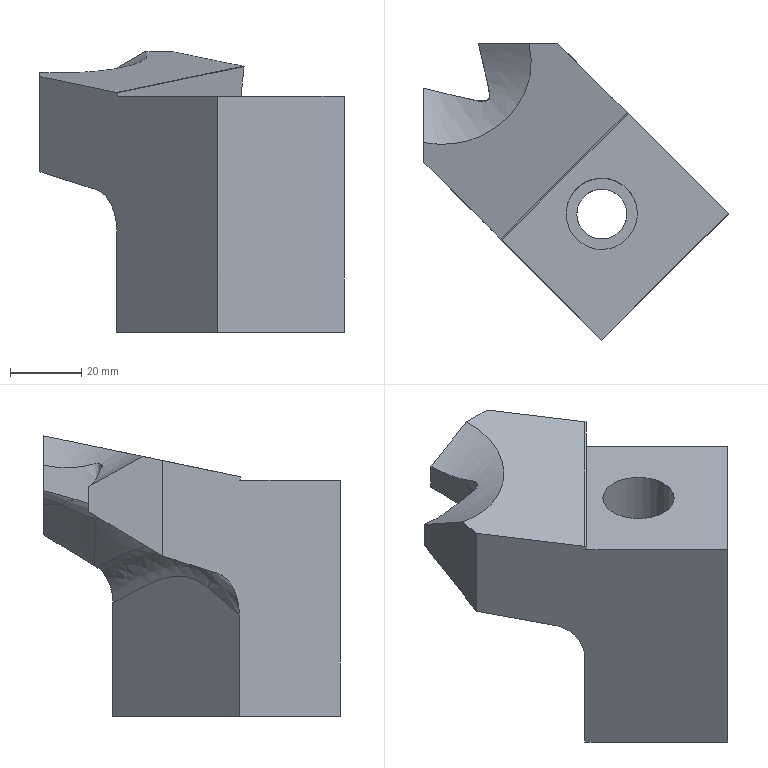Part | NX | features solid 2 | 1 solid | 28 faces | box 85.14 x 83.008 x 78.488 mm | volume 154476 mm3 | spline 16 | plane 10 | cylinder 2 | commonest cylinder face diameters 14 x1 20 x1